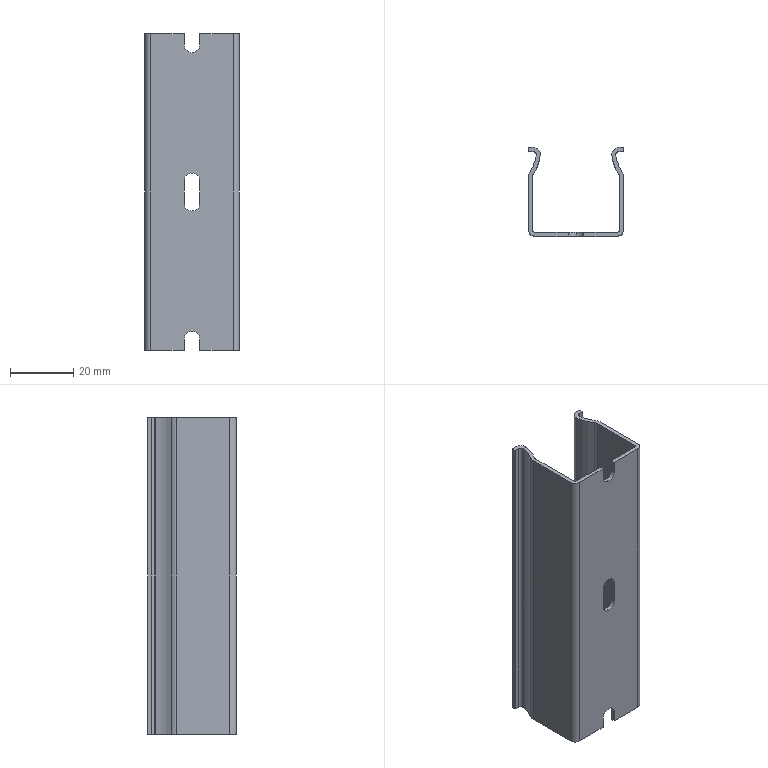Part | SolidWorks | features BaseBody 1 | 1 solid | 46 faces | box 30 x 28 x 100 mm | volume 10719 mm3 | cylinder 24 | plane 22 | commonest cylinder face diameters 5 x6 2 x3 4.5 x3 1.5 x2 3.5 x2 4 x2
STEP:
#1=CARTESIAN_POINT('',(-2.5,-14.,-100.));
#2=VERTEX_POINT('',#1);
#3=CARTESIAN_POINT('',(-2.5,-12.75,-100.));
#4=VERTEX_POINT('',#3);
#5=CARTESIAN_POINT('',(-2.5,14.001,-100.));
#6=DIRECTION('',(0.,1.,0.));
#7=VECTOR('',#6,1000.);
#8=LINE('',#5,#7);
#9=EDGE_CURVE('',#2,#4,#8,.T.);
#10=ORIENTED_EDGE('',*,*,#9,.T.);
#11=CARTESIAN_POINT('',(-2.5,-12.75,-96.5));
#12=VERTEX_POINT('',#11);
#13=CARTESIAN_POINT('',(-2.5,-12.75,-96.5));
#14=DIRECTION('',(0.,0.,1.));
#15=VECTOR('',#14,1000.);
#16=LINE('',#13,#15);
#17=EDGE_CURVE('',#4,#12,#16,.T.);
#18=ORIENTED_EDGE('',*,*,#17,.T.);
#19=CARTESIAN_POINT('',(-2.5,-14.,-96.5));
#20=VERTEX_POINT('',#19);
#21=CARTESIAN_POINT('',(-2.5,14.001,-96.5));
#22=DIRECTION('',(0.,-1.,0.));
#23=VECTOR('',#22,1000.);
#24=LINE('',#21,#23);
#25=EDGE_CURVE('',#12,#20,#24,.T.);
#26=ORIENTED_EDGE('',*,*,#25,.T.);
#27=CARTESIAN_POINT('',(-2.5,-14.,-96.5));
#28=DIRECTION('',(0.,0.,-1.));
#29=VECTOR('',#28,1000.);
#30=LINE('',#27,#29);
#31=EDGE_CURVE('',#20,#2,#30,.T.);
#32=ORIENTED_EDGE('',*,*,#31,.T.);
#33=EDGE_LOOP('',(#10,#18,#26,#32));
#34=FACE_OUTER_BOUND('',#33,.T.);
#35=CARTESIAN_POINT('',(-2.5,14.001,-96.5));
#36=DIRECTION('',(-1.,0.,0.));
#37=DIRECTION('',(0.,0.,1.));
#38=AXIS2_PLACEMENT_3D('',#35,#36,#37);
#39=PLANE('',#38);
#40=ADVANCED_FACE('',(#34),#39,.F.);
#41=CARTESIAN_POINT('',(2.5,-12.75,-100.));
#42=VERTEX_POINT('',#41);
#43=CARTESIAN_POINT('',(2.5,-14.,-100.));
#44=VERTEX_POINT('',#43);
#45=CARTESIAN_POINT('',(2.5,14.001,-100.));
#46=DIRECTION('',(0.,-1.,0.));
#47=VECTOR('',#46,1000.);
#48=LINE('',#45,#47);
#49=EDGE_CURVE('',#42,#44,#48,.T.);
#50=ORIENTED_EDGE('',*,*,#49,.T.);
#51=CARTESIAN_POINT('',(2.5,-14.,-96.5));
#52=VERTEX_POINT('',#51);
#53=CARTESIAN_POINT('',(2.5,-14.,-96.5));
#54=DIRECTION('',(0.,0.,1.));
#55=VECTOR('',#54,1000.);
#56=LINE('',#53,#55);
#57=EDGE_CURVE('',#44,#52,#56,.T.);
#58=ORIENTED_EDGE('',*,*,#57,.T.);
#59=CARTESIAN_POINT('',(2.5,-12.75,-96.5));
#60=VERTEX_POINT('',#59);
#61=CARTESIAN_POINT('',(2.5,14.001,-96.5));
#62=DIRECTION('',(0.,-1.,0.));
#63=VECTOR('',#62,1000.);
#64=LINE('',#61,#63);
#65=EDGE_CURVE('',#60,#52,#64,.T.);
#66=ORIENTED_EDGE('',*,*,#65,.F.);
#67=CARTESIAN_POINT('',(2.5,-12.75,-96.5));
#68=DIRECTION('',(0.,0.,-1.));
#69=VECTOR('',#68,1000.);
#70=LINE('',#67,#69);
#71=EDGE_CURVE('',#60,#42,#70,.T.);
#72=ORIENTED_EDGE('',*,*,#71,.T.);
#73=EDGE_LOOP('',(#50,#58,#66,#72));
#74=FACE_OUTER_BOUND('',#73,.T.);
#75=CARTESIAN_POINT('',(2.5,14.001,-96.5));
#76=DIRECTION('',(1.,0.,0.));
#77=DIRECTION('',(0.,0.,1.));
#78=AXIS2_PLACEMENT_3D('',#75,#76,#77);
#79=PLANE('',#78);
#80=ADVANCED_FACE('',(#74),#79,.F.);
#81=CARTESIAN_POINT('',(0.,-12.75,-96.5));
#82=DIRECTION('',(0.,1.,0.));
#83=DIRECTION('',(0.,0.,-1.));
#84=AXIS2_PLACEMENT_3D('',#81,#82,#83);
#85=CIRCLE('',#84,2.5);
#86=EDGE_CURVE('',#12,#60,#85,.T.);
#87=ORIENTED_EDGE('',*,*,#86,.T.);
#88=ORIENTED_EDGE('',*,*,#65,.T.);
#89=CARTESIAN_POINT('',(0.,-14.,-96.5));
#90=DIRECTION('',(0.,-1.,0.));
#91=DIRECTION('',(0.,0.,-1.));
#92=AXIS2_PLACEMENT_3D('',#89,#90,#91);
#93=CIRCLE('',#92,2.5);
#94=EDGE_CURVE('',#52,#20,#93,.T.);
#95=ORIENTED_EDGE('',*,*,#94,.T.);
#96=ORIENTED_EDGE('',*,*,#25,.F.);
#97=EDGE_LOOP('',(#87,#88,#95,#96));
#98=FACE_OUTER_BOUND('',#97,.T.);
#99=CARTESIAN_POINT('',(0.,14.001,-96.5));
#100=DIRECTION('',(0.,-1.,0.));
#101=DIRECTION('',(0.,0.,-1.));
#102=AXIS2_PLACEMENT_3D('',#99,#100,#101);
#103=CYLINDRICAL_SURFACE('',#102,2.5);
#104=ADVANCED_FACE('',(#98),#103,.F.);
#105=CARTESIAN_POINT('',(-2.5,-12.75,-53.5));
#106=VERTEX_POINT('',#105);
#107=CARTESIAN_POINT('',(-2.5,-12.75,-46.5));
#108=VERTEX_POINT('',#107);
#109=CARTESIAN_POINT('',(-2.5,-12.75,-46.5));
#110=DIRECTION('',(0.,0.,1.));
#111=VECTOR('',#110,1000.);
#112=LINE('',#109,#111);
#113=EDGE_CURVE('',#106,#108,#112,.T.);
#114=ORIENTED_EDGE('',*,*,#113,.T.);
#115=CARTESIAN_POINT('',(-2.5,-14.,-46.5));
#116=VERTEX_POINT('',#115);
#117=CARTESIAN_POINT('',(-2.5,14.001,-46.5));
#118=DIRECTION('',(0.,-1.,0.));
#119=VECTOR('',#118,1000.);
#120=LINE('',#117,#119);
#121=EDGE_CURVE('',#108,#116,#120,.T.);
#122=ORIENTED_EDGE('',*,*,#121,.T.);
#123=CARTESIAN_POINT('',(-2.5,-14.,-53.5));
#124=VERTEX_POINT('',#123);
#125=CARTESIAN_POINT('',(-2.5,-14.,-46.5));
#126=DIRECTION('',(0.,0.,-1.));
#127=VECTOR('',#126,1000.);
#128=LINE('',#125,#127);
#129=EDGE_CURVE('',#116,#124,#128,.T.);
#130=ORIENTED_EDGE('',*,*,#129,.T.);
#131=CARTESIAN_POINT('',(-2.5,14.001,-53.5));
#132=DIRECTION('',(0.,-1.,0.));
#133=VECTOR('',#132,1000.);
#134=LINE('',#131,#133);
#135=EDGE_CURVE('',#106,#124,#134,.T.);
#136=ORIENTED_EDGE('',*,*,#135,.F.);
#137=EDGE_LOOP('',(#114,#122,#130,#136));
#138=FACE_OUTER_BOUND('',#137,.T.);
#139=CARTESIAN_POINT('',(-2.5,14.001,-46.5));
#140=DIRECTION('',(-1.,0.,0.));
#141=DIRECTION('',(0.,0.,1.));
#142=AXIS2_PLACEMENT_3D('',#139,#140,#141);
#143=PLANE('',#142);
#144=ADVANCED_FACE('',(#138),#143,.F.);
#145=CARTESIAN_POINT('',(0.,-12.75,-56.));
#146=VERTEX_POINT('',#145);
#147=CARTESIAN_POINT('',(0.,-14.,-56.));
#148=VERTEX_POINT('',#147);
#149=CARTESIAN_POINT('',(0.,14.001,-56.));
#150=DIRECTION('',(0.,-1.,0.));
#151=VECTOR('',#150,1000.);
#152=LINE('',#149,#151);
#153=EDGE_CURVE('',#146,#148,#152,.T.);
#154=ORIENTED_EDGE('',*,*,#153,.F.);
#155=CARTESIAN_POINT('',(0.,-12.75,-53.5));
#156=DIRECTION('',(0.,1.,0.));
#157=DIRECTION('',(0.,0.,-1.));
#158=AXIS2_PLACEMENT_3D('',#155,#156,#157);
#159=CIRCLE('',#158,2.5);
#160=EDGE_CURVE('',#146,#106,#159,.T.);
#161=ORIENTED_EDGE('',*,*,#160,.T.);
#162=ORIENTED_EDGE('',*,*,#135,.T.);
#163=CARTESIAN_POINT('',(0.,-14.,-53.5));
#164=DIRECTION('',(0.,-1.,0.));
#165=DIRECTION('',(0.,0.,-1.));
#166=AXIS2_PLACEMENT_3D('',#163,#164,#165);
#167=CIRCLE('',#166,2.5);
#168=EDGE_CURVE('',#124,#148,#167,.T.);
#169=ORIENTED_EDGE('',*,*,#168,.T.);
#170=EDGE_LOOP('',(#154,#161,#162,#169));
#171=FACE_OUTER_BOUND('',#170,.T.);
#172=CARTESIAN_POINT('',(0.,14.001,-53.5));
#173=DIRECTION('',(0.,-1.,0.));
#174=DIRECTION('',(0.,0.,-1.));
#175=AXIS2_PLACEMENT_3D('',#172,#173,#174);
#176=CYLINDRICAL_SURFACE('',#175,2.5);
#177=ADVANCED_FACE('',(#171),#176,.F.);
#178=CARTESIAN_POINT('',(2.5,-12.75,-46.5));
#179=VERTEX_POINT('',#178);
#180=CARTESIAN_POINT('',(2.5,-12.75,-53.5));
#181=VERTEX_POINT('',#180);
#182=CARTESIAN_POINT('',(2.5,-12.75,-46.5));
#183=DIRECTION('',(0.,0.,-1.));
#184=VECTOR('',#183,1000.);
#185=LINE('',#182,#184);
#186=EDGE_CURVE('',#179,#181,#185,.T.);
#187=ORIENTED_EDGE('',*,*,#186,.T.);
#188=CARTESIAN_POINT('',(2.5,-14.,-53.5));
#189=VERTEX_POINT('',#188);
#190=CARTESIAN_POINT('',(2.5,14.001,-53.5));
#191=DIRECTION('',(0.,-1.,0.));
#192=VECTOR('',#191,1000.);
#193=LINE('',#190,#192);
#194=EDGE_CURVE('',#181,#189,#193,.T.);
#195=ORIENTED_EDGE('',*,*,#194,.T.);
#196=CARTESIAN_POINT('',(2.5,-14.,-46.5));
#197=VERTEX_POINT('',#196);
#198=CARTESIAN_POINT('',(2.5,-14.,-46.5));
#199=DIRECTION('',(0.,0.,1.));
#200=VECTOR('',#199,1000.);
#201=LINE('',#198,#200);
#202=EDGE_CURVE('',#189,#197,#201,.T.);
#203=ORIENTED_EDGE('',*,*,#202,.T.);
#204=CARTESIAN_POINT('',(2.5,14.001,-46.5));
#205=DIRECTION('',(0.,-1.,0.));
#206=VECTOR('',#205,1000.);
#207=LINE('',#204,#206);
#208=EDGE_CURVE('',#179,#197,#207,.T.);
#209=ORIENTED_EDGE('',*,*,#208,.F.);
#210=EDGE_LOOP('',(#187,#195,#203,#209));
#211=FACE_OUTER_BOUND('',#210,.T.);
#212=CARTESIAN_POINT('',(2.5,14.001,-46.5));
#213=DIRECTION('',(1.,0.,0.));
#214=DIRECTION('',(0.,0.,1.));
#215=AXIS2_PLACEMENT_3D('',#212,#213,#214);
#216=PLANE('',#215);
#217=ADVANCED_FACE('',(#211),#216,.F.);
#218=CARTESIAN_POINT('',(0.,-12.75,-46.5));
#219=DIRECTION('',(0.,1.,0.));
#220=DIRECTION('',(0.,0.,-1.));
#221=AXIS2_PLACEMENT_3D('',#218,#219,#220);
#222=CIRCLE('',#221,2.5);
#223=EDGE_CURVE('',#108,#179,#222,.T.);
#224=ORIENTED_EDGE('',*,*,#223,.T.);
#225=ORIENTED_EDGE('',*,*,#208,.T.);
#226=CARTESIAN_POINT('',(0.,-14.,-46.5));
#227=DIRECTION('',(0.,-1.,0.));
#228=DIRECTION('',(0.,0.,-1.));
#229=AXIS2_PLACEMENT_3D('',#226,#227,#228);
#230=CIRCLE('',#229,2.5);
#231=EDGE_CURVE('',#197,#116,#230,.T.);
#232=ORIENTED_EDGE('',*,*,#231,.T.);
#233=ORIENTED_EDGE('',*,*,#121,.F.);
#234=EDGE_LOOP('',(#224,#225,#232,#233));
#235=FACE_OUTER_BOUND('',#234,.T.);
#236=CARTESIAN_POINT('',(0.,14.001,-46.5));
#237=DIRECTION('',(0.,-1.,0.));
#238=DIRECTION('',(0.,0.,-1.));
#239=AXIS2_PLACEMENT_3D('',#236,#237,#238);
#240=CYLINDRICAL_SURFACE('',#239,2.5);
#241=ADVANCED_FACE('',(#235),#240,.F.);
#242=CARTESIAN_POINT('',(-2.5,-14.,0.));
#243=VERTEX_POINT('',#242);
#244=CARTESIAN_POINT('',(-2.5,-14.,-3.5));
#245=VERTEX_POINT('',#244);
#246=CARTESIAN_POINT('',(-2.5,-14.,3.5));
#247=DIRECTION('',(0.,0.,-1.));
#248=VECTOR('',#247,1000.);
#249=LINE('',#246,#248);
#250=EDGE_CURVE('',#243,#245,#249,.T.);
#251=ORIENTED_EDGE('',*,*,#250,.T.);
#252=CARTESIAN_POINT('',(-2.5,-12.75,-3.5));
#253=VERTEX_POINT('',#252);
#254=CARTESIAN_POINT('',(-2.5,14.001,-3.5));
#255=DIRECTION('',(0.,-1.,0.));
#256=VECTOR('',#255,1000.);
#257=LINE('',#254,#256);
#258=EDGE_CURVE('',#253,#245,#257,.T.);
#259=ORIENTED_EDGE('',*,*,#258,.F.);
#260=CARTESIAN_POINT('',(-2.5,-12.75,0.));
#261=VERTEX_POINT('',#260);
#262=CARTESIAN_POINT('',(-2.5,-12.75,3.5));
#263=DIRECTION('',(0.,0.,1.));
#264=VECTOR('',#263,1000.);
#265=LINE('',#262,#264);
#266=EDGE_CURVE('',#253,#261,#265,.T.);
#267=ORIENTED_EDGE('',*,*,#266,.T.);
#268=CARTESIAN_POINT('',(-2.5,14.001,0.));
#269=DIRECTION('',(0.,1.,0.));
#270=VECTOR('',#269,1000.);
#271=LINE('',#268,#270);
#272=EDGE_CURVE('',#243,#261,#271,.T.);
#273=ORIENTED_EDGE('',*,*,#272,.F.);
#274=EDGE_LOOP('',(#251,#259,#267,#273));
#275=FACE_OUTER_BOUND('',#274,.T.);
#276=CARTESIAN_POINT('',(-2.5,14.001,3.5));
#277=DIRECTION('',(-1.,0.,0.));
#278=DIRECTION('',(0.,0.,1.));
#279=AXIS2_PLACEMENT_3D('',#276,#277,#278);
#280=PLANE('',#279);
#281=ADVANCED_FACE('',(#275),#280,.F.);
#282=CARTESIAN_POINT('',(2.5,-12.75,0.));
#283=VERTEX_POINT('',#282);
#284=CARTESIAN_POINT('',(2.5,-12.75,-3.5));
#285=VERTEX_POINT('',#284);
#286=CARTESIAN_POINT('',(2.5,-12.75,3.5));
#287=DIRECTION('',(0.,0.,-1.));
#288=VECTOR('',#287,1000.);
#289=LINE('',#286,#288);
#290=EDGE_CURVE('',#283,#285,#289,.T.);
#291=ORIENTED_EDGE('',*,*,#290,.T.);
#292=CARTESIAN_POINT('',(2.5,-14.,-3.5));
#293=VERTEX_POINT('',#292);
#294=CARTESIAN_POINT('',(2.5,14.001,-3.5));
#295=DIRECTION('',(0.,-1.,0.));
#296=VECTOR('',#295,1000.);
#297=LINE('',#294,#296);
#298=EDGE_CURVE('',#285,#293,#297,.T.);
#299=ORIENTED_EDGE('',*,*,#298,.T.);
#300=CARTESIAN_POINT('',(2.5,-14.,0.));
#301=VERTEX_POINT('',#300);
#302=CARTESIAN_POINT('',(2.5,-14.,3.5));
#303=DIRECTION('',(0.,0.,1.));
#304=VECTOR('',#303,1000.);
#305=LINE('',#302,#304);
#306=EDGE_CURVE('',#293,#301,#305,.T.);
#307=ORIENTED_EDGE('',*,*,#306,.T.);
#308=CARTESIAN_POINT('',(2.5,14.001,0.));
#309=DIRECTION('',(0.,-1.,0.));
#310=VECTOR('',#309,1000.);
#311=LINE('',#308,#310);
#312=EDGE_CURVE('',#283,#301,#311,.T.);
#313=ORIENTED_EDGE('',*,*,#312,.F.);
#314=EDGE_LOOP('',(#291,#299,#307,#313));
#315=FACE_OUTER_BOUND('',#314,.T.);
#316=CARTESIAN_POINT('',(2.5,14.001,3.5));
#317=DIRECTION('',(1.,0.,0.));
#318=DIRECTION('',(0.,0.,1.));
#319=AXIS2_PLACEMENT_3D('',#316,#317,#318);
#320=PLANE('',#319);
#321=ADVANCED_FACE('',(#315),#320,.F.);
#322=CARTESIAN_POINT('',(0.,-12.75,-6.));
#323=VERTEX_POINT('',#322);
#324=CARTESIAN_POINT('',(0.,-14.,-6.));
#325=VERTEX_POINT('',#324);
#326=CARTESIAN_POINT('',(0.,14.001,-6.));
#327=DIRECTION('',(0.,-1.,0.));
#328=VECTOR('',#327,1000.);
#329=LINE('',#326,#328);
#330=EDGE_CURVE('',#323,#325,#329,.T.);
#331=ORIENTED_EDGE('',*,*,#330,.F.);
#332=CARTESIAN_POINT('',(0.,-12.75,-3.5));
#333=DIRECTION('',(0.,1.,0.));
#334=DIRECTION('',(0.,0.,-1.));
#335=AXIS2_PLACEMENT_3D('',#332,#333,#334);
#336=CIRCLE('',#335,2.5);
#337=EDGE_CURVE('',#323,#253,#336,.T.);
#338=ORIENTED_EDGE('',*,*,#337,.T.);
#339=ORIENTED_EDGE('',*,*,#258,.T.);
#340=CARTESIAN_POINT('',(0.,-14.,-3.5));
#341=DIRECTION('',(0.,-1.,0.));
#342=DIRECTION('',(0.,0.,-1.));
#343=AXIS2_PLACEMENT_3D('',#340,#341,#342);
#344=CIRCLE('',#343,2.5);
#345=EDGE_CURVE('',#245,#325,#344,.T.);
#346=ORIENTED_EDGE('',*,*,#345,.T.);
#347=EDGE_LOOP('',(#331,#338,#339,#346));
#348=FACE_OUTER_BOUND('',#347,.T.);
#349=CARTESIAN_POINT('',(0.,14.001,-3.5));
#350=DIRECTION('',(0.,-1.,0.));
#351=DIRECTION('',(0.,0.,-1.));
#352=AXIS2_PLACEMENT_3D('',#349,#350,#351);
#353=CYLINDRICAL_SURFACE('',#352,2.5);
#354=ADVANCED_FACE('',(#348),#353,.F.);
#355=CARTESIAN_POINT('',(-13.,-12.75,-100.));
#356=VERTEX_POINT('',#355);
#357=CARTESIAN_POINT('',(-13.75,-12.,-100.));
#358=VERTEX_POINT('',#357);
#359=CARTESIAN_POINT('',(-13.,-12.,-100.));
#360=DIRECTION('',(0.,0.,-1.));
#361=DIRECTION('',(1.,0.,0.));
#362=AXIS2_PLACEMENT_3D('',#359,#360,#361);
#363=CIRCLE('',#362,0.75);
#364=EDGE_CURVE('',#356,#358,#363,.T.);
#365=ORIENTED_EDGE('',*,*,#364,.T.);
#366=CARTESIAN_POINT('',(-13.75,-12.,0.));
#367=VERTEX_POINT('',#366);
#368=CARTESIAN_POINT('',(-13.75,-12.,-100.));
#369=DIRECTION('',(0.,0.,1.));
#370=VECTOR('',#369,1000.);
#371=LINE('',#368,#370);
#372=EDGE_CURVE('',#358,#367,#371,.T.);
#373=ORIENTED_EDGE('',*,*,#372,.T.);
#374=CARTESIAN_POINT('',(-13.,-12.75,0.));
#375=VERTEX_POINT('',#374);
#376=CARTESIAN_POINT('',(-13.,-12.,0.));
#377=DIRECTION('',(0.,0.,1.));
#378=DIRECTION('',(1.,0.,0.));
#379=AXIS2_PLACEMENT_3D('',#376,#377,#378);
#380=CIRCLE('',#379,0.75);
#381=EDGE_CURVE('',#367,#375,#380,.T.);
#382=ORIENTED_EDGE('',*,*,#381,.T.);
#383=CARTESIAN_POINT('',(-13.,-12.75,-100.));
#384=DIRECTION('',(0.,0.,-1.));
#385=VECTOR('',#384,1000.);
#386=LINE('',#383,#385);
#387=EDGE_CURVE('',#375,#356,#386,.T.);
#388=ORIENTED_EDGE('',*,*,#387,.T.);
#389=EDGE_LOOP('',(#365,#373,#382,#388));
#390=FACE_OUTER_BOUND('',#389,.T.);
#391=CARTESIAN_POINT('',(-13.,-12.,-100.));
#392=DIRECTION('',(0.,0.,1.));
#393=DIRECTION('',(1.,0.,0.));
#394=AXIS2_PLACEMENT_3D('',#391,#392,#393);
#395=CYLINDRICAL_SURFACE('',#394,0.75);
#396=ADVANCED_FACE('',(#390),#395,.F.);
#397=CARTESIAN_POINT('',(13.75,-12.,-100.));
#398=VERTEX_POINT('',#397);
#399=CARTESIAN_POINT('',(13.,-12.75,-100.));
#400=VERTEX_POINT('',#399);
#401=CARTESIAN_POINT('',(13.,-12.,-100.));
#402=DIRECTION('',(0.,0.,-1.));
#403=DIRECTION('',(1.,0.,0.));
#404=AXIS2_PLACEMENT_3D('',#401,#402,#403);
#405=CIRCLE('',#404,0.75);
#406=EDGE_CURVE('',#398,#400,#405,.T.);
#407=ORIENTED_EDGE('',*,*,#406,.T.);
#408=CARTESIAN_POINT('',(13.,-12.75,0.));
#409=VERTEX_POINT('',#408);
#410=CARTESIAN_POINT('',(13.,-12.75,-100.));
#411=DIRECTION('',(0.,0.,1.));
#412=VECTOR('',#411,1000.);
#413=LINE('',#410,#412);
#414=EDGE_CURVE('',#400,#409,#413,.T.);
#415=ORIENTED_EDGE('',*,*,#414,.T.);
#416=CARTESIAN_POINT('',(13.75,-12.,0.));
#417=VERTEX_POINT('',#416);
#418=CARTESIAN_POINT('',(13.,-12.,0.));
#419=DIRECTION('',(0.,0.,1.));
#420=DIRECTION('',(1.,0.,0.));
#421=AXIS2_PLACEMENT_3D('',#418,#419,#420);
#422=CIRCLE('',#421,0.75);
#423=EDGE_CURVE('',#409,#417,#422,.T.);
#424=ORIENTED_EDGE('',*,*,#423,.T.);
#425=CARTESIAN_POINT('',(13.75,-12.,-100.));
#426=DIRECTION('',(0.,0.,-1.));
#427=VECTOR('',#426,1000.);
#428=LINE('',#425,#427);
#429=EDGE_CURVE('',#417,#398,#428,.T.);
#430=ORIENTED_EDGE('',*,*,#429,.T.);
#431=EDGE_LOOP('',(#407,#415,#424,#430));
#432=FACE_OUTER_BOUND('',#431,.T.);
#433=CARTESIAN_POINT('',(13.,-12.,-100.));
#434=DIRECTION('',(0.,0.,1.));
#435=DIRECTION('',(1.,0.,0.));
#436=AXIS2_PLACEMENT_3D('',#433,#434,#435);
#437=CYLINDRICAL_SURFACE('',#436,0.75);
#438=ADVANCED_FACE('',(#432),#437,.F.);
#439=CARTESIAN_POINT('',(13.439,5.746,-100.));
#440=VERTEX_POINT('',#439);
#441=CARTESIAN_POINT('',(13.75,4.75,-100.));
#442=VERTEX_POINT('',#441);
#443=CARTESIAN_POINT('',(12.,4.75,-100.));
#444=DIRECTION('',(0.,0.,-1.));
#445=DIRECTION('',(1.,0.,0.));
#446=AXIS2_PLACEMENT_3D('',#443,#444,#445);
#447=CIRCLE('',#446,1.75);
#448=EDGE_CURVE('',#440,#442,#447,.T.);
#449=ORIENTED_EDGE('',*,*,#448,.T.);
#450=CARTESIAN_POINT('',(13.75,4.75,0.));
#451=VERTEX_POINT('',#450);
#452=CARTESIAN_POINT('',(13.75,4.75,-100.));
#453=DIRECTION('',(0.,0.,1.));
#454=VECTOR('',#453,1000.);
#455=LINE('',#452,#454);
#456=EDGE_CURVE('',#442,#451,#455,.T.);
#457=ORIENTED_EDGE('',*,*,#456,.T.);
#458=CARTESIAN_POINT('',(13.439,5.746,0.));
#459=VERTEX_POINT('',#458);
#460=CARTESIAN_POINT('',(12.,4.75,0.));
#461=DIRECTION('',(0.,0.,1.));
#462=DIRECTION('',(1.,0.,0.));
#463=AXIS2_PLACEMENT_3D('',#460,#461,#462);
#464=CIRCLE('',#463,1.75);
#465=EDGE_CURVE('',#451,#459,#464,.T.);
#466=ORIENTED_EDGE('',*,*,#465,.T.);
#467=CARTESIAN_POINT('',(13.439,5.746,-100.));
#468=DIRECTION('',(0.,0.,-1.));
#469=VECTOR('',#468,1000.);
#470=LINE('',#467,#469);
#471=EDGE_CURVE('',#459,#440,#470,.T.);
#472=ORIENTED_EDGE('',*,*,#471,.T.);
#473=EDGE_LOOP('',(#449,#457,#466,#472));
#474=FACE_OUTER_BOUND('',#473,.T.);
#475=CARTESIAN_POINT('',(12.,4.75,-100.));
#476=DIRECTION('',(0.,0.,1.));
#477=DIRECTION('',(1.,0.,0.));
#478=AXIS2_PLACEMENT_3D('',#475,#476,#477);
#479=CYLINDRICAL_SURFACE('',#478,1.75);
#480=ADVANCED_FACE('',(#474),#479,.F.);
#481=CARTESIAN_POINT('',(-13.75,4.75,-100.));
#482=VERTEX_POINT('',#481);
#483=CARTESIAN_POINT('',(-13.439,5.746,-100.));
#484=VERTEX_POINT('',#483);
#485=CARTESIAN_POINT('',(-12.,4.75,-100.));
#486=DIRECTION('',(0.,0.,-1.));
#487=DIRECTION('',(1.,0.,0.));
#488=AXIS2_PLACEMENT_3D('',#485,#486,#487);
#489=CIRCLE('',#488,1.75);
#490=EDGE_CURVE('',#482,#484,#489,.T.);
#491=ORIENTED_EDGE('',*,*,#490,.T.);
#492=CARTESIAN_POINT('',(-13.439,5.746,0.));
#493=VERTEX_POINT('',#492);
#494=CARTESIAN_POINT('',(-13.439,5.746,-100.));
#495=DIRECTION('',(0.,0.,1.));
#496=VECTOR('',#495,1000.);
#497=LINE('',#494,#496);
#498=EDGE_CURVE('',#484,#493,#497,.T.);
#499=ORIENTED_EDGE('',*,*,#498,.T.);
#500=CARTESIAN_POINT('',(-13.75,4.75,0.));
#501=VERTEX_POINT('',#500);
#502=CARTESIAN_POINT('',(-12.,4.75,0.));
#503=DIRECTION('',(0.,0.,1.));
#504=DIRECTION('',(1.,0.,0.));
#505=AXIS2_PLACEMENT_3D('',#502,#503,#504);
#506=CIRCLE('',#505,1.75);
#507=EDGE_CURVE('',#493,#501,#506,.T.);
#508=ORIENTED_EDGE('',*,*,#507,.T.);
#509=CARTESIAN_POINT('',(-13.75,4.75,-100.));
#510=DIRECTION('',(0.,0.,-1.));
#511=VECTOR('',#510,1000.);
#512=LINE('',#509,#511);
#513=EDGE_CURVE('',#501,#482,#512,.T.);
#514=ORIENTED_EDGE('',*,*,#513,.T.);
#515=EDGE_LOOP('',(#491,#499,#508,#514));
#516=FACE_OUTER_BOUND('',#515,.T.);
#517=CARTESIAN_POINT('',(-12.,4.75,-100.));
#518=DIRECTION('',(0.,0.,1.));
#519=DIRECTION('',(1.,0.,0.));
#520=AXIS2_PLACEMENT_3D('',#517,#518,#519);
#521=CYLINDRICAL_SURFACE('',#520,1.75);
#522=ADVANCED_FACE('',(#516),#521,.F.);
#523=CARTESIAN_POINT('',(13.55,14.,-100.));
#524=VERTEX_POINT('',#523);
#525=CARTESIAN_POINT('',(11.311,11.526,-100.));
#526=VERTEX_POINT('',#525);
#527=CARTESIAN_POINT('',(13.55,11.75,-100.));
#528=DIRECTION('',(0.,0.,1.));
#529=DIRECTION('',(1.,0.,0.));
#530=AXIS2_PLACEMENT_3D('',#527,#528,#529);
#531=CIRCLE('',#530,2.25);
#532=EDGE_CURVE('',#524,#526,#531,.T.);
#533=ORIENTED_EDGE('',*,*,#532,.T.);
#534=CARTESIAN_POINT('',(11.311,11.526,0.));
#535=VERTEX_POINT('',#534);
#536=CARTESIAN_POINT('',(11.311,11.526,-100.));
#537=DIRECTION('',(0.,0.,1.));
#538=VECTOR('',#537,1000.);
#539=LINE('',#536,#538);
#540=EDGE_CURVE('',#526,#535,#539,.T.);
#541=ORIENTED_EDGE('',*,*,#540,.T.);
#542=CARTESIAN_POINT('',(13.55,14.,0.));
#543=VERTEX_POINT('',#542);
#544=CARTESIAN_POINT('',(13.55,11.75,0.));
#545=DIRECTION('',(0.,0.,-1.));
#546=DIRECTION('',(1.,0.,0.));
#547=AXIS2_PLACEMENT_3D('',#544,#545,#546);
#548=CIRCLE('',#547,2.25);
#549=EDGE_CURVE('',#535,#543,#548,.T.);
#550=ORIENTED_EDGE('',*,*,#549,.T.);
#551=CARTESIAN_POINT('',(13.55,14.,-100.));
#552=DIRECTION('',(0.,0.,-1.));
#553=VECTOR('',#552,1000.);
#554=LINE('',#551,#553);
#555=EDGE_CURVE('',#543,#524,#554,.T.);
#556=ORIENTED_EDGE('',*,*,#555,.T.);
#557=EDGE_LOOP('',(#533,#541,#550,#556));
#558=FACE_OUTER_BOUND('',#557,.T.);
#559=CARTESIAN_POINT('',(13.55,11.75,-100.));
#560=DIRECTION('',(0.,0.,1.));
#561=DIRECTION('',(1.,0.,0.));
#562=AXIS2_PLACEMENT_3D('',#559,#560,#561);
#563=CYLINDRICAL_SURFACE('',#562,2.25);
#564=ADVANCED_FACE('',(#558),#563,.T.);
#565=CARTESIAN_POINT('',(-11.3,11.75,-100.));
#566=VERTEX_POINT('',#565);
#567=CARTESIAN_POINT('',(-11.3,11.75,0.));
#568=VERTEX_POINT('',#567);
#569=CARTESIAN_POINT('',(-11.3,11.75,-100.));
#570=DIRECTION('',(0.,0.,1.));
#571=VECTOR('',#570,1000.);
#572=LINE('',#569,#571);
#573=EDGE_CURVE('',#566,#568,#572,.T.);
#574=ORIENTED_EDGE('',*,*,#573,.F.);
#575=CARTESIAN_POINT('',(-13.55,14.,-100.));
#576=VERTEX_POINT('',#575);
#577=CARTESIAN_POINT('',(-13.55,11.75,-100.));
#578=DIRECTION('',(0.,0.,1.));
#579=DIRECTION('',(1.,0.,0.));
#580=AXIS2_PLACEMENT_3D('',#577,#578,#579);
#581=CIRCLE('',#580,2.25);
#582=EDGE_CURVE('',#566,#576,#581,.T.);
#583=ORIENTED_EDGE('',*,*,#582,.T.);
#584=CARTESIAN_POINT('',(-13.55,14.,0.));
#585=VERTEX_POINT('',#584);
#586=CARTESIAN_POINT('',(-13.55,14.,-100.));
#587=DIRECTION('',(0.,0.,1.));
#588=VECTOR('',#587,1000.);
#589=LINE('',#586,#588);
#590=EDGE_CURVE('',#576,#585,#589,.T.);
#591=ORIENTED_EDGE('',*,*,#590,.T.);
#592=CARTESIAN_POINT('',(-13.55,11.75,0.));
#593=DIRECTION('',(0.,0.,-1.));
#594=DIRECTION('',(1.,0.,0.));
#595=AXIS2_PLACEMENT_3D('',#592,#593,#594);
#596=CIRCLE('',#595,2.25);
#597=EDGE_CURVE('',#585,#568,#596,.T.);
#598=ORIENTED_EDGE('',*,*,#597,.T.);
#599=EDGE_LOOP('',(#574,#583,#591,#598));
#600=FACE_OUTER_BOUND('',#599,.T.);
#601=CARTESIAN_POINT('',(-13.55,11.75,-100.));
#602=DIRECTION('',(0.,0.,1.));
#603=DIRECTION('',(1.,0.,0.));
#604=AXIS2_PLACEMENT_3D('',#601,#602,#603);
#605=CYLINDRICAL_SURFACE('',#604,2.25);
#606=ADVANCED_FACE('',(#600),#605,.T.);
#607=CARTESIAN_POINT('',(-11.311,11.526,-100.));
#608=VERTEX_POINT('',#607);
#609=CARTESIAN_POINT('',(-23.55,12.75,-100.));
#610=DIRECTION('',(0.,0.,1.));
#611=DIRECTION('',(1.,0.,0.));
#612=AXIS2_PLACEMENT_3D('',#609,#610,#611);
#613=CIRCLE('',#612,12.3);
#614=EDGE_CURVE('',#484,#608,#613,.T.);
#615=ORIENTED_EDGE('',*,*,#614,.T.);
#616=CARTESIAN_POINT('',(-11.311,11.526,0.));
#617=VERTEX_POINT('',#616);
#618=CARTESIAN_POINT('',(-11.311,11.526,-100.));
#619=DIRECTION('',(0.,0.,-1.));
#620=VECTOR('',#619,1000.);
#621=LINE('',#618,#620);
#622=EDGE_CURVE('',#617,#608,#621,.T.);
#623=ORIENTED_EDGE('',*,*,#622,.F.);
#624=CARTESIAN_POINT('',(-23.55,12.75,0.));
#625=DIRECTION('',(0.,0.,1.));
#626=DIRECTION('',(1.,0.,0.));
#627=AXIS2_PLACEMENT_3D('',#624,#625,#626);
#628=CIRCLE('',#627,12.3);
#629=EDGE_CURVE('',#493,#617,#628,.T.);
#630=ORIENTED_EDGE('',*,*,#629,.F.);
#631=ORIENTED_EDGE('',*,*,#498,.F.);
#632=EDGE_LOOP('',(#615,#623,#630,#631));
#633=FACE_OUTER_BOUND('',#632,.T.);
#634=CARTESIAN_POINT('',(-23.55,12.75,-100.));
#635=DIRECTION('',(0.,0.,1.));
#636=DIRECTION('',(1.,0.,0.));
#637=AXIS2_PLACEMENT_3D('',#634,#635,#636);
#638=CYLINDRICAL_SURFACE('',#637,12.3);
#639=ADVANCED_FACE('',(#633),#638,.T.);
#640=CARTESIAN_POINT('',(23.55,12.75,0.));
#641=DIRECTION('',(0.,0.,1.));
#642=DIRECTION('',(1.,0.,0.));
#643=AXIS2_PLACEMENT_3D('',#640,#641,#642);
#644=CIRCLE('',#643,12.3);
#645=EDGE_CURVE('',#535,#459,#644,.T.);
#646=ORIENTED_EDGE('',*,*,#645,.F.);
#647=ORIENTED_EDGE('',*,*,#540,.F.);
#648=CARTESIAN_POINT('',(23.55,12.75,-100.));
#649=DIRECTION('',(0.,0.,1.));
#650=DIRECTION('',(1.,0.,0.));
#651=AXIS2_PLACEMENT_3D('',#648,#649,#650);
#652=CIRCLE('',#651,12.3);
#653=EDGE_CURVE('',#526,#440,#652,.T.);
#654=ORIENTED_EDGE('',*,*,#653,.T.);
#655=ORIENTED_EDGE('',*,*,#471,.F.);
#656=EDGE_LOOP('',(#646,#647,#654,#655));
#657=FACE_OUTER_BOUND('',#656,.T.);
#658=CARTESIAN_POINT('',(23.55,12.75,-100.));
#659=DIRECTION('',(0.,0.,1.));
#660=DIRECTION('',(1.,0.,0.));
#661=AXIS2_PLACEMENT_3D('',#658,#659,#660);
#662=CYLINDRICAL_SURFACE('',#661,12.3);
#663=ADVANCED_FACE('',(#657),#662,.T.);
#664=ORIENTED_EDGE('',*,*,#186,.F.);
#665=ORIENTED_EDGE('',*,*,#223,.F.);
#666=ORIENTED_EDGE('',*,*,#113,.F.);
#667=ORIENTED_EDGE('',*,*,#160,.F.);
#668=CARTESIAN_POINT('',(0.,-12.75,-53.5));
#669=DIRECTION('',(0.,1.,0.));
#670=DIRECTION('',(0.,0.,-1.));
#671=AXIS2_PLACEMENT_3D('',#668,#669,#670);
#672=CIRCLE('',#671,2.5);
#673=EDGE_CURVE('',#181,#146,#672,.T.);
#674=ORIENTED_EDGE('',*,*,#673,.F.);
#675=EDGE_LOOP('',(#664,#665,#666,#667,#674));
#676=FACE_BOUND('',#675,.T.);
#677=CARTESIAN_POINT('',(0.,-12.75,-100.));
#678=DIRECTION('',(1.,0.,0.));
#679=VECTOR('',#678,1000.);
#680=LINE('',#677,#679);
#681=EDGE_CURVE('',#42,#400,#680,.T.);
#682=ORIENTED_EDGE('',*,*,#681,.F.);
#683=ORIENTED_EDGE('',*,*,#71,.F.);
#684=ORIENTED_EDGE('',*,*,#86,.F.);
#685=ORIENTED_EDGE('',*,*,#17,.F.);
#686=CARTESIAN_POINT('',(0.,-12.75,-100.));
#687=DIRECTION('',(1.,0.,0.));
#688=VECTOR('',#687,1000.);
#689=LINE('',#686,#688);
#690=EDGE_CURVE('',#356,#4,#689,.T.);
#691=ORIENTED_EDGE('',*,*,#690,.F.);
#692=ORIENTED_EDGE('',*,*,#387,.F.);
#693=CARTESIAN_POINT('',(0.,-12.75,0.));
#694=DIRECTION('',(1.,0.,0.));
#695=VECTOR('',#694,1000.);
#696=LINE('',#693,#695);
#697=EDGE_CURVE('',#375,#261,#696,.T.);
#698=ORIENTED_EDGE('',*,*,#697,.T.);
#699=ORIENTED_EDGE('',*,*,#266,.F.);
#700=ORIENTED_EDGE('',*,*,#337,.F.);
#701=CARTESIAN_POINT('',(0.,-12.75,-3.5));
#702=DIRECTION('',(0.,1.,0.));
#703=DIRECTION('',(0.,0.,-1.));
#704=AXIS2_PLACEMENT_3D('',#701,#702,#703);
#705=CIRCLE('',#704,2.5);
#706=EDGE_CURVE('',#285,#323,#705,.T.);
#707=ORIENTED_EDGE('',*,*,#706,.F.);
#708=ORIENTED_EDGE('',*,*,#290,.F.);
#709=CARTESIAN_POINT('',(0.,-12.75,0.));
#710=DIRECTION('',(1.,0.,0.));
#711=VECTOR('',#710,1000.);
#712=LINE('',#709,#711);
#713=EDGE_CURVE('',#283,#409,#712,.T.);
#714=ORIENTED_EDGE('',*,*,#713,.T.);
#715=ORIENTED_EDGE('',*,*,#414,.F.);
#716=EDGE_LOOP('',(#682,#683,#684,#685,#691,#692,#698,#699,#700,#707,#708,#714,#715));
#717=FACE_OUTER_BOUND('',#716,.T.);
#718=CARTESIAN_POINT('',(-15.,-12.75,-100.));
#719=DIRECTION('',(0.,-1.,0.));
#720=DIRECTION('',(0.,0.,-1.));
#721=AXIS2_PLACEMENT_3D('',#718,#719,#720);
#722=PLANE('',#721);
#723=ADVANCED_FACE('',(#676,#717),#722,.F.);
#724=CARTESIAN_POINT('',(13.75,0.,0.));
#725=DIRECTION('',(0.,1.,0.));
#726=VECTOR('',#725,1000.);
#727=LINE('',#724,#726);
#728=EDGE_CURVE('',#417,#451,#727,.T.);
#729=ORIENTED_EDGE('',*,*,#728,.T.);
#730=ORIENTED_EDGE('',*,*,#456,.F.);
#731=CARTESIAN_POINT('',(13.75,0.,-100.));
#732=DIRECTION('',(0.,1.,0.));
#733=VECTOR('',#732,1000.);
#734=LINE('',#731,#733);
#735=EDGE_CURVE('',#398,#442,#734,.T.);
#736=ORIENTED_EDGE('',*,*,#735,.F.);
#737=ORIENTED_EDGE('',*,*,#429,.F.);
#738=EDGE_LOOP('',(#729,#730,#736,#737));
#739=FACE_OUTER_BOUND('',#738,.T.);
#740=CARTESIAN_POINT('',(13.75,14.,-100.));
#741=DIRECTION('',(1.,0.,0.));
#742=DIRECTION('',(0.,1.,0.));
#743=AXIS2_PLACEMENT_3D('',#740,#741,#742);
#744=PLANE('',#743);
#745=ADVANCED_FACE('',(#739),#744,.F.);
#746=CARTESIAN_POINT('',(-13.75,0.,-100.));
#747=DIRECTION('',(0.,-1.,0.));
#748=VECTOR('',#747,1000.);
#749=LINE('',#746,#748);
#750=EDGE_CURVE('',#482,#358,#749,.T.);
#751=ORIENTED_EDGE('',*,*,#750,.F.);
#752=ORIENTED_EDGE('',*,*,#513,.F.);
#753=CARTESIAN_POINT('',(-13.75,0.,0.));
#754=DIRECTION('',(0.,-1.,0.));
#755=VECTOR('',#754,1000.);
#756=LINE('',#753,#755);
#757=EDGE_CURVE('',#501,#367,#756,.T.);
#758=ORIENTED_EDGE('',*,*,#757,.T.);
#759=ORIENTED_EDGE('',*,*,#372,.F.);
#760=EDGE_LOOP('',(#751,#752,#758,#759));
#761=FACE_OUTER_BOUND('',#760,.T.);
#762=CARTESIAN_POINT('',(-13.75,14.,-100.));
#763=DIRECTION('',(-1.,0.,0.));
#764=DIRECTION('',(0.,1.,0.));
#765=AXIS2_PLACEMENT_3D('',#762,#763,#764);
#766=PLANE('',#765);
#767=ADVANCED_FACE('',(#761),#766,.F.);
#768=CARTESIAN_POINT('',(-13.,-14.,-100.));
#769=VERTEX_POINT('',#768);
#770=CARTESIAN_POINT('',(-15.,-12.,-100.));
#771=VERTEX_POINT('',#770);
#772=CARTESIAN_POINT('',(-13.,-12.,-100.));
#773=DIRECTION('',(0.,0.,-1.));
#774=DIRECTION('',(1.,0.,0.));
#775=AXIS2_PLACEMENT_3D('',#772,#773,#774);
#776=CIRCLE('',#775,2.);
#777=EDGE_CURVE('',#769,#771,#776,.T.);
#778=ORIENTED_EDGE('',*,*,#777,.F.);
#779=CARTESIAN_POINT('',(-13.,-14.,0.));
#780=VERTEX_POINT('',#779);
#781=CARTESIAN_POINT('',(-13.,-14.,-100.));
#782=DIRECTION('',(0.,0.,-1.));
#783=VECTOR('',#782,1000.);
#784=LINE('',#781,#783);
#785=EDGE_CURVE('',#780,#769,#784,.T.);
#786=ORIENTED_EDGE('',*,*,#785,.F.);
#787=CARTESIAN_POINT('',(-15.,-12.,0.));
#788=VERTEX_POINT('',#787);
#789=CARTESIAN_POINT('',(-13.,-12.,0.));
#790=DIRECTION('',(0.,0.,1.));
#791=DIRECTION('',(1.,0.,0.));
#792=AXIS2_PLACEMENT_3D('',#789,#790,#791);
#793=CIRCLE('',#792,2.);
#794=EDGE_CURVE('',#788,#780,#793,.T.);
#795=ORIENTED_EDGE('',*,*,#794,.F.);
#796=CARTESIAN_POINT('',(-15.,-12.,-100.));
#797=DIRECTION('',(0.,0.,1.));
#798=VECTOR('',#797,1000.);
#799=LINE('',#796,#798);
#800=EDGE_CURVE('',#771,#788,#799,.T.);
#801=ORIENTED_EDGE('',*,*,#800,.F.);
#802=EDGE_LOOP('',(#778,#786,#795,#801));
#803=FACE_OUTER_BOUND('',#802,.T.);
#804=CARTESIAN_POINT('',(-13.,-12.,-100.));
#805=DIRECTION('',(0.,0.,1.));
#806=DIRECTION('',(1.,0.,0.));
#807=AXIS2_PLACEMENT_3D('',#804,#805,#806);
#808=CYLINDRICAL_SURFACE('',#807,2.);
#809=ADVANCED_FACE('',(#803),#808,.T.);
#810=CARTESIAN_POINT('',(15.,-12.,-100.));
#811=VERTEX_POINT('',#810);
#812=CARTESIAN_POINT('',(13.,-14.,-100.));
#813=VERTEX_POINT('',#812);
#814=CARTESIAN_POINT('',(13.,-12.,-100.));
#815=DIRECTION('',(0.,0.,-1.));
#816=DIRECTION('',(1.,0.,0.));
#817=AXIS2_PLACEMENT_3D('',#814,#815,#816);
#818=CIRCLE('',#817,2.);
#819=EDGE_CURVE('',#811,#813,#818,.T.);
#820=ORIENTED_EDGE('',*,*,#819,.F.);
#821=CARTESIAN_POINT('',(15.,-12.,0.));
#822=VERTEX_POINT('',#821);
#823=CARTESIAN_POINT('',(15.,-12.,-100.));
#824=DIRECTION('',(0.,0.,-1.));
#825=VECTOR('',#824,1000.);
#826=LINE('',#823,#825);
#827=EDGE_CURVE('',#822,#811,#826,.T.);
#828=ORIENTED_EDGE('',*,*,#827,.F.);
#829=CARTESIAN_POINT('',(13.,-14.,0.));
#830=VERTEX_POINT('',#829);
#831=CARTESIAN_POINT('',(13.,-12.,0.));
#832=DIRECTION('',(0.,0.,1.));
#833=DIRECTION('',(1.,0.,0.));
#834=AXIS2_PLACEMENT_3D('',#831,#832,#833);
#835=CIRCLE('',#834,2.);
#836=EDGE_CURVE('',#830,#822,#835,.T.);
#837=ORIENTED_EDGE('',*,*,#836,.F.);
#838=CARTESIAN_POINT('',(13.,-14.,-100.));
#839=DIRECTION('',(0.,0.,1.));
#840=VECTOR('',#839,1000.);
#841=LINE('',#838,#840);
#842=EDGE_CURVE('',#813,#830,#841,.T.);
#843=ORIENTED_EDGE('',*,*,#842,.F.);
#844=EDGE_LOOP('',(#820,#828,#837,#843));
#845=FACE_OUTER_BOUND('',#844,.T.);
#846=CARTESIAN_POINT('',(13.,-12.,-100.));
#847=DIRECTION('',(0.,0.,1.));
#848=DIRECTION('',(1.,0.,0.));
#849=AXIS2_PLACEMENT_3D('',#846,#847,#848);
#850=CYLINDRICAL_SURFACE('',#849,2.);
#851=ADVANCED_FACE('',(#845),#850,.T.);
#852=CARTESIAN_POINT('',(14.466,6.458,-100.));
#853=VERTEX_POINT('',#852);
#854=CARTESIAN_POINT('',(15.,4.75,-100.));
#855=VERTEX_POINT('',#854);
#856=CARTESIAN_POINT('',(12.,4.75,-100.));
#857=DIRECTION('',(0.,0.,-1.));
#858=DIRECTION('',(1.,0.,0.));
#859=AXIS2_PLACEMENT_3D('',#856,#857,#858);
#860=CIRCLE('',#859,3.);
#861=EDGE_CURVE('',#853,#855,#860,.T.);
#862=ORIENTED_EDGE('',*,*,#861,.F.);
#863=CARTESIAN_POINT('',(14.466,6.458,0.));
#864=VERTEX_POINT('',#863);
#865=CARTESIAN_POINT('',(14.466,6.458,-100.));
#866=DIRECTION('',(0.,0.,-1.));
#867=VECTOR('',#866,1000.);
#868=LINE('',#865,#867);
#869=EDGE_CURVE('',#864,#853,#868,.T.);
#870=ORIENTED_EDGE('',*,*,#869,.F.);
#871=CARTESIAN_POINT('',(15.,4.75,0.));
#872=VERTEX_POINT('',#871);
#873=CARTESIAN_POINT('',(12.,4.75,0.));
#874=DIRECTION('',(0.,0.,1.));
#875=DIRECTION('',(1.,0.,0.));
#876=AXIS2_PLACEMENT_3D('',#873,#874,#875);
#877=CIRCLE('',#876,3.);
#878=EDGE_CURVE('',#872,#864,#877,.T.);
#879=ORIENTED_EDGE('',*,*,#878,.F.);
#880=CARTESIAN_POINT('',(15.,4.75,0.));
#881=DIRECTION('',(0.,0.,1.));
#882=VECTOR('',#881,1000.);
#883=LINE('',#880,#882);
#884=EDGE_CURVE('',#855,#872,#883,.T.);
#885=ORIENTED_EDGE('',*,*,#884,.F.);
#886=EDGE_LOOP('',(#862,#870,#879,#885));
#887=FACE_OUTER_BOUND('',#886,.T.);
#888=CARTESIAN_POINT('',(12.,4.75,-100.));
#889=DIRECTION('',(0.,0.,1.));
#890=DIRECTION('',(1.,0.,0.));
#891=AXIS2_PLACEMENT_3D('',#888,#889,#890);
#892=CYLINDRICAL_SURFACE('',#891,3.);
#893=ADVANCED_FACE('',(#887),#892,.T.);
#894=CARTESIAN_POINT('',(-15.,4.75,-100.));
#895=VERTEX_POINT('',#894);
#896=CARTESIAN_POINT('',(-14.466,6.458,-100.));
#897=VERTEX_POINT('',#896);
#898=CARTESIAN_POINT('',(-12.,4.75,-100.));
#899=DIRECTION('',(0.,0.,-1.));
#900=DIRECTION('',(1.,0.,0.));
#901=AXIS2_PLACEMENT_3D('',#898,#899,#900);
#902=CIRCLE('',#901,3.);
#903=EDGE_CURVE('',#895,#897,#902,.T.);
#904=ORIENTED_EDGE('',*,*,#903,.F.);
#905=CARTESIAN_POINT('',(-15.,4.75,0.));
#906=VERTEX_POINT('',#905);
#907=CARTESIAN_POINT('',(-15.,4.75,-100.));
#908=DIRECTION('',(0.,0.,-1.));
#909=VECTOR('',#908,1000.);
#910=LINE('',#907,#909);
#911=EDGE_CURVE('',#906,#895,#910,.T.);
#912=ORIENTED_EDGE('',*,*,#911,.F.);
#913=CARTESIAN_POINT('',(-14.466,6.458,0.));
#914=VERTEX_POINT('',#913);
#915=CARTESIAN_POINT('',(-12.,4.75,0.));
#916=DIRECTION('',(0.,0.,1.));
#917=DIRECTION('',(1.,0.,0.));
#918=AXIS2_PLACEMENT_3D('',#915,#916,#917);
#919=CIRCLE('',#918,3.);
#920=EDGE_CURVE('',#914,#906,#919,.T.);
#921=ORIENTED_EDGE('',*,*,#920,.F.);
#922=CARTESIAN_POINT('',(-14.466,6.458,-100.));
#923=DIRECTION('',(0.,0.,1.));
#924=VECTOR('',#923,1000.);
#925=LINE('',#922,#924);
#926=EDGE_CURVE('',#897,#914,#925,.T.);
#927=ORIENTED_EDGE('',*,*,#926,.F.);
#928=EDGE_LOOP('',(#904,#912,#921,#927));
#929=FACE_OUTER_BOUND('',#928,.T.);
#930=CARTESIAN_POINT('',(-12.,4.75,-100.));
#931=DIRECTION('',(0.,0.,1.));
#932=DIRECTION('',(1.,0.,0.));
#933=AXIS2_PLACEMENT_3D('',#930,#931,#932);
#934=CYLINDRICAL_SURFACE('',#933,3.);
#935=ADVANCED_FACE('',(#929),#934,.T.);
#936=CARTESIAN_POINT('',(13.55,12.75,-100.));
#937=VERTEX_POINT('',#936);
#938=CARTESIAN_POINT('',(12.555,11.65,-100.));
#939=VERTEX_POINT('',#938);
#940=CARTESIAN_POINT('',(13.55,11.75,-100.));
#941=DIRECTION('',(0.,0.,1.));
#942=DIRECTION('',(1.,0.,0.));
#943=AXIS2_PLACEMENT_3D('',#940,#941,#942);
#944=CIRCLE('',#943,1.);
#945=EDGE_CURVE('',#937,#939,#944,.T.);
#946=ORIENTED_EDGE('',*,*,#945,.F.);
#947=CARTESIAN_POINT('',(13.55,12.75,0.));
#948=VERTEX_POINT('',#947);
#949=CARTESIAN_POINT('',(13.55,12.75,-100.));
#950=DIRECTION('',(0.,0.,-1.));
#951=VECTOR('',#950,1000.);
#952=LINE('',#949,#951);
#953=EDGE_CURVE('',#948,#937,#952,.T.);
#954=ORIENTED_EDGE('',*,*,#953,.F.);
#955=CARTESIAN_POINT('',(12.555,11.65,0.));
#956=VERTEX_POINT('',#955);
#957=CARTESIAN_POINT('',(13.55,11.75,0.));
#958=DIRECTION('',(0.,0.,-1.));
#959=DIRECTION('',(1.,0.,0.));
#960=AXIS2_PLACEMENT_3D('',#957,#958,#959);
#961=CIRCLE('',#960,1.);
#962=EDGE_CURVE('',#956,#948,#961,.T.);
#963=ORIENTED_EDGE('',*,*,#962,.F.);
#964=CARTESIAN_POINT('',(12.555,11.65,-100.));
#965=DIRECTION('',(0.,0.,1.));
#966=VECTOR('',#965,1000.);
#967=LINE('',#964,#966);
#968=EDGE_CURVE('',#939,#956,#967,.T.);
#969=ORIENTED_EDGE('',*,*,#968,.F.);
#970=EDGE_LOOP('',(#946,#954,#963,#969));
#971=FACE_OUTER_BOUND('',#970,.T.);
#972=CARTESIAN_POINT('',(13.55,11.75,-100.));
#973=DIRECTION('',(0.,0.,1.));
#974=DIRECTION('',(1.,0.,0.));
#975=AXIS2_PLACEMENT_3D('',#972,#973,#974);
#976=CYLINDRICAL_SURFACE('',#975,1.);
#977=ADVANCED_FACE('',(#971),#976,.F.);
#978=CARTESIAN_POINT('',(-12.55,11.75,-100.));
#979=VERTEX_POINT('',#978);
#980=CARTESIAN_POINT('',(-12.55,11.75,0.));
#981=VERTEX_POINT('',#980);
#982=CARTESIAN_POINT('',(-12.55,11.75,-100.));
#983=DIRECTION('',(0.,0.,1.));
#984=VECTOR('',#983,1000.);
#985=LINE('',#982,#984);
#986=EDGE_CURVE('',#979,#981,#985,.T.);
#987=ORIENTED_EDGE('',*,*,#986,.F.);
#988=CARTESIAN_POINT('',(-12.555,11.65,-100.));
#989=VERTEX_POINT('',#988);
#990=CARTESIAN_POINT('',(-13.55,11.75,-100.));
#991=DIRECTION('',(0.,0.,1.));
#992=DIRECTION('',(1.,0.,0.));
#993=AXIS2_PLACEMENT_3D('',#990,#991,#992);
#994=CIRCLE('',#993,1.);
#995=EDGE_CURVE('',#989,#979,#994,.T.);
#996=ORIENTED_EDGE('',*,*,#995,.F.);
#997=CARTESIAN_POINT('',(-12.555,11.65,0.));
#998=VERTEX_POINT('',#997);
#999=CARTESIAN_POINT('',(-12.555,11.65,-100.));
#1000=DIRECTION('',(0.,0.,-1.));
#1001=VECTOR('',#1000,1000.);
#1002=LINE('',#999,#1001);
#1003=EDGE_CURVE('',#998,#989,#1002,.T.);
#1004=ORIENTED_EDGE('',*,*,#1003,.F.);
#1005=CARTESIAN_POINT('',(-13.55,11.75,0.));
#1006=DIRECTION('',(0.,0.,-1.));
#1007=DIRECTION('',(1.,0.,0.));
#1008=AXIS2_PLACEMENT_3D('',#1005,#1006,#1007);
#1009=CIRCLE('',#1008,1.);
#1010=EDGE_CURVE('',#981,#998,#1009,.T.);
#1011=ORIENTED_EDGE('',*,*,#1010,.F.);
#1012=EDGE_LOOP('',(#987,#996,#1004,#1011));
#1013=FACE_OUTER_BOUND('',#1012,.T.);
#1014=CARTESIAN_POINT('',(-13.55,11.75,-100.));
#1015=DIRECTION('',(0.,0.,1.));
#1016=DIRECTION('',(1.,0.,0.));
#1017=AXIS2_PLACEMENT_3D('',#1014,#1015,#1016);
#1018=CYLINDRICAL_SURFACE('',#1017,1.);
#1019=ADVANCED_FACE('',(#1013),#1018,.F.);
#1020=CARTESIAN_POINT('',(-13.55,12.75,-100.));
#1021=VERTEX_POINT('',#1020);
#1022=CARTESIAN_POINT('',(-15.,12.75,-100.));
#1023=VERTEX_POINT('',#1022);
#1024=CARTESIAN_POINT('',(-15.,12.75,-100.));
#1025=DIRECTION('',(-1.,0.,0.));
#1026=VECTOR('',#1025,1000.);
#1027=LINE('',#1024,#1026);
#1028=EDGE_CURVE('',#1021,#1023,#1027,.T.);
#1029=ORIENTED_EDGE('',*,*,#1028,.F.);
#1030=CARTESIAN_POINT('',(-13.55,12.75,0.));
#1031=VERTEX_POINT('',#1030);
#1032=CARTESIAN_POINT('',(-13.55,12.75,0.));
#1033=DIRECTION('',(0.,0.,1.));
#1034=VECTOR('',#1033,1000.);
#1035=LINE('',#1032,#1034);
#1036=EDGE_CURVE('',#1021,#1031,#1035,.T.);
#1037=ORIENTED_EDGE('',*,*,#1036,.T.);
#1038=CARTESIAN_POINT('',(-15.,12.75,0.));
#1039=VERTEX_POINT('',#1038);
#1040=CARTESIAN_POINT('',(-15.,12.75,0.));
#1041=DIRECTION('',(-1.,0.,0.));
#1042=VECTOR('',#1041,1000.);
#1043=LINE('',#1040,#1042);
#1044=EDGE_CURVE('',#1031,#1039,#1043,.T.);
#1045=ORIENTED_EDGE('',*,*,#1044,.T.);
#1046=CARTESIAN_POINT('',(-15.,12.75,-100.));
#1047=DIRECTION('',(0.,0.,1.));
#1048=VECTOR('',#1047,1000.);
#1049=LINE('',#1046,#1048);
#1050=EDGE_CURVE('',#1023,#1039,#1049,.T.);
#1051=ORIENTED_EDGE('',*,*,#1050,.F.);
#1052=EDGE_LOOP('',(#1029,#1037,#1045,#1051));
#1053=FACE_OUTER_BOUND('',#1052,.T.);
#1054=CARTESIAN_POINT('',(-15.,12.75,-100.));
#1055=DIRECTION('',(0.,1.,0.));
#1056=DIRECTION('',(1.,0.,0.));
#1057=AXIS2_PLACEMENT_3D('',#1054,#1055,#1056);
#1058=PLANE('',#1057);
#1059=ADVANCED_FACE('',(#1053),#1058,.F.);
#1060=CARTESIAN_POINT('',(-23.55,12.75,-100.));
#1061=DIRECTION('',(0.,0.,1.));
#1062=DIRECTION('',(-1.,0.,0.));
#1063=AXIS2_PLACEMENT_3D('',#1060,#1061,#1062);
#1064=CIRCLE('',#1063,11.05);
#1065=EDGE_CURVE('',#897,#989,#1064,.T.);
#1066=ORIENTED_EDGE('',*,*,#1065,.F.);
#1067=ORIENTED_EDGE('',*,*,#926,.T.);
#1068=CARTESIAN_POINT('',(-23.55,12.75,0.));
#1069=DIRECTION('',(0.,0.,1.));
#1070=DIRECTION('',(-1.,0.,0.));
#1071=AXIS2_PLACEMENT_3D('',#1068,#1069,#1070);
#1072=CIRCLE('',#1071,11.05);
#1073=EDGE_CURVE('',#914,#998,#1072,.T.);
#1074=ORIENTED_EDGE('',*,*,#1073,.T.);
#1075=ORIENTED_EDGE('',*,*,#1003,.T.);
#1076=EDGE_LOOP('',(#1066,#1067,#1074,#1075));
#1077=FACE_OUTER_BOUND('',#1076,.T.);
#1078=CARTESIAN_POINT('',(-23.55,12.75,-100.));
#1079=DIRECTION('',(0.,0.,1.));
#1080=DIRECTION('',(1.,0.,0.));
#1081=AXIS2_PLACEMENT_3D('',#1078,#1079,#1080);
#1082=CYLINDRICAL_SURFACE('',#1081,11.05);
#1083=ADVANCED_FACE('',(#1077),#1082,.F.);
#1084=CARTESIAN_POINT('',(15.,12.75,0.));
#1085=VERTEX_POINT('',#1084);
#1086=CARTESIAN_POINT('',(15.,12.75,0.));
#1087=DIRECTION('',(-1.,0.,0.));
#1088=VECTOR('',#1087,1000.);
#1089=LINE('',#1086,#1088);
#1090=EDGE_CURVE('',#1085,#948,#1089,.T.);
#1091=ORIENTED_EDGE('',*,*,#1090,.T.);
#1092=ORIENTED_EDGE('',*,*,#953,.T.);
#1093=CARTESIAN_POINT('',(15.,12.75,-100.));
#1094=VERTEX_POINT('',#1093);
#1095=CARTESIAN_POINT('',(15.,12.75,-100.));
#1096=DIRECTION('',(-1.,0.,0.));
#1097=VECTOR('',#1096,1000.);
#1098=LINE('',#1095,#1097);
#1099=EDGE_CURVE('',#1094,#937,#1098,.T.);
#1100=ORIENTED_EDGE('',*,*,#1099,.F.);
#1101=CARTESIAN_POINT('',(15.,12.75,-100.));
#1102=DIRECTION('',(0.,0.,1.));
#1103=VECTOR('',#1102,1000.);
#1104=LINE('',#1101,#1103);
#1105=EDGE_CURVE('',#1094,#1085,#1104,.T.);
#1106=ORIENTED_EDGE('',*,*,#1105,.T.);
#1107=EDGE_LOOP('',(#1091,#1092,#1100,#1106));
#1108=FACE_OUTER_BOUND('',#1107,.T.);
#1109=CARTESIAN_POINT('',(15.,12.75,-100.));
#1110=DIRECTION('',(0.,1.,0.));
#1111=DIRECTION('',(1.,0.,0.));
#1112=AXIS2_PLACEMENT_3D('',#1109,#1110,#1111);
#1113=PLANE('',#1112);
#1114=ADVANCED_FACE('',(#1108),#1113,.F.);
#1115=CARTESIAN_POINT('',(23.55,12.75,0.));
#1116=DIRECTION('',(0.,0.,1.));
#1117=DIRECTION('',(1.,0.,0.));
#1118=AXIS2_PLACEMENT_3D('',#1115,#1116,#1117);
#1119=CIRCLE('',#1118,11.05);
#1120=EDGE_CURVE('',#956,#864,#1119,.T.);
#1121=ORIENTED_EDGE('',*,*,#1120,.T.);
#1122=ORIENTED_EDGE('',*,*,#869,.T.);
#1123=CARTESIAN_POINT('',(23.55,12.75,-100.));
#1124=DIRECTION('',(0.,0.,1.));
#1125=DIRECTION('',(1.,0.,0.));
#1126=AXIS2_PLACEMENT_3D('',#1123,#1124,#1125);
#1127=CIRCLE('',#1126,11.05);
#1128=EDGE_CURVE('',#939,#853,#1127,.T.);
#1129=ORIENTED_EDGE('',*,*,#1128,.F.);
#1130=ORIENTED_EDGE('',*,*,#968,.T.);
#1131=EDGE_LOOP('',(#1121,#1122,#1129,#1130));
#1132=FACE_OUTER_BOUND('',#1131,.T.);
#1133=CARTESIAN_POINT('',(23.55,12.75,-100.));
#1134=DIRECTION('',(0.,0.,1.));
#1135=DIRECTION('',(1.,0.,0.));
#1136=AXIS2_PLACEMENT_3D('',#1133,#1134,#1135);
#1137=CYLINDRICAL_SURFACE('',#1136,11.05);
#1138=ADVANCED_FACE('',(#1132),#1137,.F.);
#1139=ORIENTED_EDGE('',*,*,#272,.T.);
#1140=ORIENTED_EDGE('',*,*,#697,.F.);
#1141=ORIENTED_EDGE('',*,*,#381,.F.);
#1142=ORIENTED_EDGE('',*,*,#757,.F.);
#1143=ORIENTED_EDGE('',*,*,#507,.F.);
#1144=ORIENTED_EDGE('',*,*,#629,.T.);
#1145=CARTESIAN_POINT('',(-13.55,11.75,0.));
#1146=DIRECTION('',(0.,0.,-1.));
#1147=DIRECTION('',(1.,0.,0.));
#1148=AXIS2_PLACEMENT_3D('',#1145,#1146,#1147);
#1149=CIRCLE('',#1148,2.25);
#1150=EDGE_CURVE('',#568,#617,#1149,.T.);
#1151=ORIENTED_EDGE('',*,*,#1150,.F.);
#1152=ORIENTED_EDGE('',*,*,#597,.F.);
#1153=CARTESIAN_POINT('',(-15.,14.,0.));
#1154=VERTEX_POINT('',#1153);
#1155=CARTESIAN_POINT('',(-15.,14.,0.));
#1156=DIRECTION('',(-1.,0.,0.));
#1157=VECTOR('',#1156,1000.);
#1158=LINE('',#1155,#1157);
#1159=EDGE_CURVE('',#585,#1154,#1158,.T.);
#1160=ORIENTED_EDGE('',*,*,#1159,.T.);
#1161=CARTESIAN_POINT('',(-15.,14.,0.));
#1162=DIRECTION('',(0.,-1.,0.));
#1163=VECTOR('',#1162,1000.);
#1164=LINE('',#1161,#1163);
#1165=EDGE_CURVE('',#1154,#1039,#1164,.T.);
#1166=ORIENTED_EDGE('',*,*,#1165,.T.);
#1167=ORIENTED_EDGE('',*,*,#1044,.F.);
#1168=CARTESIAN_POINT('',(-13.55,11.75,0.));
#1169=DIRECTION('',(0.,0.,-1.));
#1170=DIRECTION('',(1.,0.,0.));
#1171=AXIS2_PLACEMENT_3D('',#1168,#1169,#1170);
#1172=CIRCLE('',#1171,1.);
#1173=EDGE_CURVE('',#1031,#981,#1172,.T.);
#1174=ORIENTED_EDGE('',*,*,#1173,.T.);
#1175=ORIENTED_EDGE('',*,*,#1010,.T.);
#1176=ORIENTED_EDGE('',*,*,#1073,.F.);
#1177=ORIENTED_EDGE('',*,*,#920,.T.);
#1178=CARTESIAN_POINT('',(-15.,14.,0.));
#1179=DIRECTION('',(0.,-1.,0.));
#1180=VECTOR('',#1179,1000.);
#1181=LINE('',#1178,#1180);
#1182=EDGE_CURVE('',#906,#788,#1181,.T.);
#1183=ORIENTED_EDGE('',*,*,#1182,.T.);
#1184=ORIENTED_EDGE('',*,*,#794,.T.);
#1185=CARTESIAN_POINT('',(-15.,-14.,0.));
#1186=DIRECTION('',(1.,0.,0.));
#1187=VECTOR('',#1186,1000.);
#1188=LINE('',#1185,#1187);
#1189=EDGE_CURVE('',#780,#243,#1188,.T.);
#1190=ORIENTED_EDGE('',*,*,#1189,.T.);
#1191=EDGE_LOOP('',(#1139,#1140,#1141,#1142,#1143,#1144,#1151,#1152,#1160,#1166,#1167,#1174,#1175,#1176,#1177,#1183,#1184,#1190));
#1192=FACE_OUTER_BOUND('',#1191,.T.);
#1193=CARTESIAN_POINT('',(0.,0.,0.));
#1194=DIRECTION('',(0.,0.,1.));
#1195=DIRECTION('',(1.,0.,0.));
#1196=AXIS2_PLACEMENT_3D('',#1193,#1194,#1195);
#1197=PLANE('',#1196);
#1198=ADVANCED_FACE('',(#1192),#1197,.T.);
#1199=ORIENTED_EDGE('',*,*,#555,.F.);
#1200=CARTESIAN_POINT('',(15.,14.,0.));
#1201=VERTEX_POINT('',#1200);
#1202=CARTESIAN_POINT('',(-15.,14.,0.));
#1203=DIRECTION('',(-1.,0.,0.));
#1204=VECTOR('',#1203,1000.);
#1205=LINE('',#1202,#1204);
#1206=EDGE_CURVE('',#1201,#543,#1205,.T.);
#1207=ORIENTED_EDGE('',*,*,#1206,.F.);
#1208=CARTESIAN_POINT('',(15.,14.,-100.));
#1209=VERTEX_POINT('',#1208);
#1210=CARTESIAN_POINT('',(15.,14.,-100.));
#1211=DIRECTION('',(0.,0.,1.));
#1212=VECTOR('',#1211,1000.);
#1213=LINE('',#1210,#1212);
#1214=EDGE_CURVE('',#1209,#1201,#1213,.T.);
#1215=ORIENTED_EDGE('',*,*,#1214,.F.);
#1216=CARTESIAN_POINT('',(-15.,14.,-100.));
#1217=DIRECTION('',(-1.,0.,0.));
#1218=VECTOR('',#1217,1000.);
#1219=LINE('',#1216,#1218);
#1220=EDGE_CURVE('',#1209,#524,#1219,.T.);
#1221=ORIENTED_EDGE('',*,*,#1220,.T.);
#1222=EDGE_LOOP('',(#1199,#1207,#1215,#1221));
#1223=FACE_OUTER_BOUND('',#1222,.T.);
#1224=CARTESIAN_POINT('',(-15.,14.,-100.));
#1225=DIRECTION('',(0.,1.,0.));
#1226=DIRECTION('',(1.,0.,0.));
#1227=AXIS2_PLACEMENT_3D('',#1224,#1225,#1226);
#1228=PLANE('',#1227);
#1229=ADVANCED_FACE('',(#1223),#1228,.T.);
#1230=ORIENTED_EDGE('',*,*,#1050,.T.);
#1231=ORIENTED_EDGE('',*,*,#1165,.F.);
#1232=CARTESIAN_POINT('',(-15.,14.,-100.));
#1233=VERTEX_POINT('',#1232);
#1234=CARTESIAN_POINT('',(-15.,14.,-100.));
#1235=DIRECTION('',(0.,0.,1.));
#1236=VECTOR('',#1235,1000.);
#1237=LINE('',#1234,#1236);
#1238=EDGE_CURVE('',#1233,#1154,#1237,.T.);
#1239=ORIENTED_EDGE('',*,*,#1238,.F.);
#1240=CARTESIAN_POINT('',(-15.,14.,-100.));
#1241=DIRECTION('',(0.,-1.,0.));
#1242=VECTOR('',#1241,1000.);
#1243=LINE('',#1240,#1242);
#1244=EDGE_CURVE('',#1233,#1023,#1243,.T.);
#1245=ORIENTED_EDGE('',*,*,#1244,.T.);
#1246=EDGE_LOOP('',(#1230,#1231,#1239,#1245));
#1247=FACE_OUTER_BOUND('',#1246,.T.);
#1248=CARTESIAN_POINT('',(-15.,14.,-100.));
#1249=DIRECTION('',(-1.,0.,0.));
#1250=DIRECTION('',(0.,1.,0.));
#1251=AXIS2_PLACEMENT_3D('',#1248,#1249,#1250);
#1252=PLANE('',#1251);
#1253=ADVANCED_FACE('',(#1247),#1252,.T.);
#1254=ORIENTED_EDGE('',*,*,#231,.F.);
#1255=ORIENTED_EDGE('',*,*,#202,.F.);
#1256=CARTESIAN_POINT('',(0.,-14.,-53.5));
#1257=DIRECTION('',(0.,-1.,0.));
#1258=DIRECTION('',(0.,0.,-1.));
#1259=AXIS2_PLACEMENT_3D('',#1256,#1257,#1258);
#1260=CIRCLE('',#1259,2.5);
#1261=EDGE_CURVE('',#148,#189,#1260,.T.);
#1262=ORIENTED_EDGE('',*,*,#1261,.F.);
#1263=ORIENTED_EDGE('',*,*,#168,.F.);
#1264=ORIENTED_EDGE('',*,*,#129,.F.);
#1265=EDGE_LOOP('',(#1254,#1255,#1262,#1263,#1264));
#1266=FACE_BOUND('',#1265,.T.);
#1267=ORIENTED_EDGE('',*,*,#57,.F.);
#1268=CARTESIAN_POINT('',(-15.,-14.,-100.));
#1269=DIRECTION('',(1.,0.,0.));
#1270=VECTOR('',#1269,1000.);
#1271=LINE('',#1268,#1270);
#1272=EDGE_CURVE('',#44,#813,#1271,.T.);
#1273=ORIENTED_EDGE('',*,*,#1272,.T.);
#1274=ORIENTED_EDGE('',*,*,#842,.T.);
#1275=CARTESIAN_POINT('',(-15.,-14.,0.));
#1276=DIRECTION('',(1.,0.,0.));
#1277=VECTOR('',#1276,1000.);
#1278=LINE('',#1275,#1277);
#1279=EDGE_CURVE('',#301,#830,#1278,.T.);
#1280=ORIENTED_EDGE('',*,*,#1279,.F.);
#1281=ORIENTED_EDGE('',*,*,#306,.F.);
#1282=CARTESIAN_POINT('',(0.,-14.,-3.5));
#1283=DIRECTION('',(0.,-1.,0.));
#1284=DIRECTION('',(0.,0.,-1.));
#1285=AXIS2_PLACEMENT_3D('',#1282,#1283,#1284);
#1286=CIRCLE('',#1285,2.5);
#1287=EDGE_CURVE('',#325,#293,#1286,.T.);
#1288=ORIENTED_EDGE('',*,*,#1287,.F.);
#1289=ORIENTED_EDGE('',*,*,#345,.F.);
#1290=ORIENTED_EDGE('',*,*,#250,.F.);
#1291=ORIENTED_EDGE('',*,*,#1189,.F.);
#1292=ORIENTED_EDGE('',*,*,#785,.T.);
#1293=CARTESIAN_POINT('',(-15.,-14.,-100.));
#1294=DIRECTION('',(1.,0.,0.));
#1295=VECTOR('',#1294,1000.);
#1296=LINE('',#1293,#1295);
#1297=EDGE_CURVE('',#769,#2,#1296,.T.);
#1298=ORIENTED_EDGE('',*,*,#1297,.T.);
#1299=ORIENTED_EDGE('',*,*,#31,.F.);
#1300=ORIENTED_EDGE('',*,*,#94,.F.);
#1301=EDGE_LOOP('',(#1267,#1273,#1274,#1280,#1281,#1288,#1289,#1290,#1291,#1292,#1298,#1299,#1300));
#1302=FACE_OUTER_BOUND('',#1301,.T.);
#1303=CARTESIAN_POINT('',(-15.,-14.,-100.));
#1304=DIRECTION('',(0.,-1.,0.));
#1305=DIRECTION('',(0.,0.,-1.));
#1306=AXIS2_PLACEMENT_3D('',#1303,#1304,#1305);
#1307=PLANE('',#1306);
#1308=ADVANCED_FACE('',(#1266,#1302),#1307,.T.);
#1309=ORIENTED_EDGE('',*,*,#1105,.F.);
#1310=CARTESIAN_POINT('',(15.,14.,-100.));
#1311=DIRECTION('',(0.,1.,0.));
#1312=VECTOR('',#1311,1000.);
#1313=LINE('',#1310,#1312);
#1314=EDGE_CURVE('',#1094,#1209,#1313,.T.);
#1315=ORIENTED_EDGE('',*,*,#1314,.T.);
#1316=ORIENTED_EDGE('',*,*,#1214,.T.);
#1317=CARTESIAN_POINT('',(15.,14.,0.));
#1318=DIRECTION('',(0.,1.,0.));
#1319=VECTOR('',#1318,1000.);
#1320=LINE('',#1317,#1319);
#1321=EDGE_CURVE('',#1085,#1201,#1320,.T.);
#1322=ORIENTED_EDGE('',*,*,#1321,.F.);
#1323=EDGE_LOOP('',(#1309,#1315,#1316,#1322));
#1324=FACE_OUTER_BOUND('',#1323,.T.);
#1325=CARTESIAN_POINT('',(15.,14.,-100.));
#1326=DIRECTION('',(1.,0.,0.));
#1327=DIRECTION('',(0.,1.,0.));
#1328=AXIS2_PLACEMENT_3D('',#1325,#1326,#1327);
#1329=PLANE('',#1328);
#1330=ADVANCED_FACE('',(#1324),#1329,.T.);
#1331=CARTESIAN_POINT('',(15.,14.,0.));
#1332=DIRECTION('',(0.,1.,0.));
#1333=VECTOR('',#1332,1000.);
#1334=LINE('',#1331,#1333);
#1335=EDGE_CURVE('',#822,#872,#1334,.T.);
#1336=ORIENTED_EDGE('',*,*,#1335,.F.);
#1337=ORIENTED_EDGE('',*,*,#827,.T.);
#1338=CARTESIAN_POINT('',(15.,14.,-100.));
#1339=DIRECTION('',(0.,1.,0.));
#1340=VECTOR('',#1339,1000.);
#1341=LINE('',#1338,#1340);
#1342=EDGE_CURVE('',#811,#855,#1341,.T.);
#1343=ORIENTED_EDGE('',*,*,#1342,.T.);
#1344=ORIENTED_EDGE('',*,*,#884,.T.);
#1345=EDGE_LOOP('',(#1336,#1337,#1343,#1344));
#1346=FACE_OUTER_BOUND('',#1345,.T.);
#1347=CARTESIAN_POINT('',(15.,14.,-100.));
#1348=DIRECTION('',(1.,0.,0.));
#1349=DIRECTION('',(0.,1.,0.));
#1350=AXIS2_PLACEMENT_3D('',#1347,#1348,#1349);
#1351=PLANE('',#1350);
#1352=ADVANCED_FACE('',(#1346),#1351,.T.);
#1353=CARTESIAN_POINT('',(-15.,14.,-100.));
#1354=DIRECTION('',(0.,-1.,0.));
#1355=VECTOR('',#1354,1000.);
#1356=LINE('',#1353,#1355);
#1357=EDGE_CURVE('',#895,#771,#1356,.T.);
#1358=ORIENTED_EDGE('',*,*,#1357,.T.);
#1359=ORIENTED_EDGE('',*,*,#800,.T.);
#1360=ORIENTED_EDGE('',*,*,#1182,.F.);
#1361=ORIENTED_EDGE('',*,*,#911,.T.);
#1362=EDGE_LOOP('',(#1358,#1359,#1360,#1361));
#1363=FACE_OUTER_BOUND('',#1362,.T.);
#1364=CARTESIAN_POINT('',(-15.,14.,-100.));
#1365=DIRECTION('',(-1.,0.,0.));
#1366=DIRECTION('',(0.,1.,0.));
#1367=AXIS2_PLACEMENT_3D('',#1364,#1365,#1366);
#1368=PLANE('',#1367);
#1369=ADVANCED_FACE('',(#1363),#1368,.T.);
#1370=ORIENTED_EDGE('',*,*,#690,.T.);
#1371=ORIENTED_EDGE('',*,*,#9,.F.);
#1372=ORIENTED_EDGE('',*,*,#1297,.F.);
#1373=ORIENTED_EDGE('',*,*,#777,.T.);
#1374=ORIENTED_EDGE('',*,*,#1357,.F.);
#1375=ORIENTED_EDGE('',*,*,#903,.T.);
#1376=ORIENTED_EDGE('',*,*,#1065,.T.);
#1377=ORIENTED_EDGE('',*,*,#995,.T.);
#1378=CARTESIAN_POINT('',(-13.55,11.75,-100.));
#1379=DIRECTION('',(0.,0.,1.));
#1380=DIRECTION('',(1.,0.,0.));
#1381=AXIS2_PLACEMENT_3D('',#1378,#1379,#1380);
#1382=CIRCLE('',#1381,1.);
#1383=EDGE_CURVE('',#979,#1021,#1382,.T.);
#1384=ORIENTED_EDGE('',*,*,#1383,.T.);
#1385=ORIENTED_EDGE('',*,*,#1028,.T.);
#1386=ORIENTED_EDGE('',*,*,#1244,.F.);
#1387=CARTESIAN_POINT('',(-15.,14.,-100.));
#1388=DIRECTION('',(-1.,0.,0.));
#1389=VECTOR('',#1388,1000.);
#1390=LINE('',#1387,#1389);
#1391=EDGE_CURVE('',#576,#1233,#1390,.T.);
#1392=ORIENTED_EDGE('',*,*,#1391,.F.);
#1393=ORIENTED_EDGE('',*,*,#582,.F.);
#1394=CARTESIAN_POINT('',(-13.55,11.75,-100.));
#1395=DIRECTION('',(0.,0.,1.));
#1396=DIRECTION('',(1.,0.,0.));
#1397=AXIS2_PLACEMENT_3D('',#1394,#1395,#1396);
#1398=CIRCLE('',#1397,2.25);
#1399=EDGE_CURVE('',#608,#566,#1398,.T.);
#1400=ORIENTED_EDGE('',*,*,#1399,.F.);
#1401=ORIENTED_EDGE('',*,*,#614,.F.);
#1402=ORIENTED_EDGE('',*,*,#490,.F.);
#1403=ORIENTED_EDGE('',*,*,#750,.T.);
#1404=ORIENTED_EDGE('',*,*,#364,.F.);
#1405=EDGE_LOOP('',(#1370,#1371,#1372,#1373,#1374,#1375,#1376,#1377,#1384,#1385,#1386,#1392,#1393,#1400,#1401,#1402,#1403,#1404));
#1406=FACE_OUTER_BOUND('',#1405,.T.);
#1407=CARTESIAN_POINT('',(0.,0.,-100.));
#1408=DIRECTION('',(0.,0.,1.));
#1409=DIRECTION('',(1.,0.,0.));
#1410=AXIS2_PLACEMENT_3D('',#1407,#1408,#1409);
#1411=PLANE('',#1410);
#1412=ADVANCED_FACE('',(#1406),#1411,.F.);
#1413=ORIENTED_EDGE('',*,*,#590,.F.);
#1414=ORIENTED_EDGE('',*,*,#1391,.T.);
#1415=ORIENTED_EDGE('',*,*,#1238,.T.);
#1416=ORIENTED_EDGE('',*,*,#1159,.F.);
#1417=EDGE_LOOP('',(#1413,#1414,#1415,#1416));
#1418=FACE_OUTER_BOUND('',#1417,.T.);
#1419=CARTESIAN_POINT('',(-15.,14.,-100.));
#1420=DIRECTION('',(0.,1.,0.));
#1421=DIRECTION('',(1.,0.,0.));
#1422=AXIS2_PLACEMENT_3D('',#1419,#1420,#1421);
#1423=PLANE('',#1422);
#1424=ADVANCED_FACE('',(#1418),#1423,.T.);
#1425=ORIENTED_EDGE('',*,*,#312,.T.);
#1426=ORIENTED_EDGE('',*,*,#1279,.T.);
#1427=ORIENTED_EDGE('',*,*,#836,.T.);
#1428=ORIENTED_EDGE('',*,*,#1335,.T.);
#1429=ORIENTED_EDGE('',*,*,#878,.T.);
#1430=ORIENTED_EDGE('',*,*,#1120,.F.);
#1431=ORIENTED_EDGE('',*,*,#962,.T.);
#1432=ORIENTED_EDGE('',*,*,#1090,.F.);
#1433=ORIENTED_EDGE('',*,*,#1321,.T.);
#1434=ORIENTED_EDGE('',*,*,#1206,.T.);
#1435=ORIENTED_EDGE('',*,*,#549,.F.);
#1436=ORIENTED_EDGE('',*,*,#645,.T.);
#1437=ORIENTED_EDGE('',*,*,#465,.F.);
#1438=ORIENTED_EDGE('',*,*,#728,.F.);
#1439=ORIENTED_EDGE('',*,*,#423,.F.);
#1440=ORIENTED_EDGE('',*,*,#713,.F.);
#1441=EDGE_LOOP('',(#1425,#1426,#1427,#1428,#1429,#1430,#1431,#1432,#1433,#1434,#1435,#1436,#1437,#1438,#1439,#1440));
#1442=FACE_OUTER_BOUND('',#1441,.T.);
#1443=CARTESIAN_POINT('',(0.,0.,0.));
#1444=DIRECTION('',(0.,0.,1.));
#1445=DIRECTION('',(1.,0.,0.));
#1446=AXIS2_PLACEMENT_3D('',#1443,#1444,#1445);
#1447=PLANE('',#1446);
#1448=ADVANCED_FACE('',(#1442),#1447,.T.);
#1449=ORIENTED_EDGE('',*,*,#1272,.F.);
#1450=ORIENTED_EDGE('',*,*,#49,.F.);
#1451=ORIENTED_EDGE('',*,*,#681,.T.);
#1452=ORIENTED_EDGE('',*,*,#406,.F.);
#1453=ORIENTED_EDGE('',*,*,#735,.T.);
#1454=ORIENTED_EDGE('',*,*,#448,.F.);
#1455=ORIENTED_EDGE('',*,*,#653,.F.);
#1456=ORIENTED_EDGE('',*,*,#532,.F.);
#1457=ORIENTED_EDGE('',*,*,#1220,.F.);
#1458=ORIENTED_EDGE('',*,*,#1314,.F.);
#1459=ORIENTED_EDGE('',*,*,#1099,.T.);
#1460=ORIENTED_EDGE('',*,*,#945,.T.);
#1461=ORIENTED_EDGE('',*,*,#1128,.T.);
#1462=ORIENTED_EDGE('',*,*,#861,.T.);
#1463=ORIENTED_EDGE('',*,*,#1342,.F.);
#1464=ORIENTED_EDGE('',*,*,#819,.T.);
#1465=EDGE_LOOP('',(#1449,#1450,#1451,#1452,#1453,#1454,#1455,#1456,#1457,#1458,#1459,#1460,#1461,#1462,#1463,#1464));
#1466=FACE_OUTER_BOUND('',#1465,.T.);
#1467=CARTESIAN_POINT('',(0.,0.,-100.));
#1468=DIRECTION('',(0.,0.,1.));
#1469=DIRECTION('',(1.,0.,0.));
#1470=AXIS2_PLACEMENT_3D('',#1467,#1468,#1469);
#1471=PLANE('',#1470);
#1472=ADVANCED_FACE('',(#1466),#1471,.F.);
#1473=ORIENTED_EDGE('',*,*,#1383,.F.);
#1474=ORIENTED_EDGE('',*,*,#986,.T.);
#1475=ORIENTED_EDGE('',*,*,#1173,.F.);
#1476=ORIENTED_EDGE('',*,*,#1036,.F.);
#1477=EDGE_LOOP('',(#1473,#1474,#1475,#1476));
#1478=FACE_OUTER_BOUND('',#1477,.T.);
#1479=CARTESIAN_POINT('',(-13.55,11.75,-100.));
#1480=DIRECTION('',(0.,0.,1.));
#1481=DIRECTION('',(1.,0.,0.));
#1482=AXIS2_PLACEMENT_3D('',#1479,#1480,#1481);
#1483=CYLINDRICAL_SURFACE('',#1482,1.);
#1484=ADVANCED_FACE('',(#1478),#1483,.F.);
#1485=ORIENTED_EDGE('',*,*,#1399,.T.);
#1486=ORIENTED_EDGE('',*,*,#573,.T.);
#1487=ORIENTED_EDGE('',*,*,#1150,.T.);
#1488=ORIENTED_EDGE('',*,*,#622,.T.);
#1489=EDGE_LOOP('',(#1485,#1486,#1487,#1488));
#1490=FACE_OUTER_BOUND('',#1489,.T.);
#1491=CARTESIAN_POINT('',(-13.55,11.75,-100.));
#1492=DIRECTION('',(0.,0.,1.));
#1493=DIRECTION('',(1.,0.,0.));
#1494=AXIS2_PLACEMENT_3D('',#1491,#1492,#1493);
#1495=CYLINDRICAL_SURFACE('',#1494,2.25);
#1496=ADVANCED_FACE('',(#1490),#1495,.T.);
#1497=ORIENTED_EDGE('',*,*,#706,.T.);
#1498=ORIENTED_EDGE('',*,*,#330,.T.);
#1499=ORIENTED_EDGE('',*,*,#1287,.T.);
#1500=ORIENTED_EDGE('',*,*,#298,.F.);
#1501=EDGE_LOOP('',(#1497,#1498,#1499,#1500));
#1502=FACE_OUTER_BOUND('',#1501,.T.);
#1503=CARTESIAN_POINT('',(0.,14.001,-3.5));
#1504=DIRECTION('',(0.,-1.,0.));
#1505=DIRECTION('',(0.,0.,-1.));
#1506=AXIS2_PLACEMENT_3D('',#1503,#1504,#1505);
#1507=CYLINDRICAL_SURFACE('',#1506,2.5);
#1508=ADVANCED_FACE('',(#1502),#1507,.F.);
#1509=ORIENTED_EDGE('',*,*,#673,.T.);
#1510=ORIENTED_EDGE('',*,*,#153,.T.);
#1511=ORIENTED_EDGE('',*,*,#1261,.T.);
#1512=ORIENTED_EDGE('',*,*,#194,.F.);
#1513=EDGE_LOOP('',(#1509,#1510,#1511,#1512));
#1514=FACE_OUTER_BOUND('',#1513,.T.);
#1515=CARTESIAN_POINT('',(0.,14.001,-53.5));
#1516=DIRECTION('',(0.,-1.,0.));
#1517=DIRECTION('',(0.,0.,-1.));
#1518=AXIS2_PLACEMENT_3D('',#1515,#1516,#1517);
#1519=CYLINDRICAL_SURFACE('',#1518,2.5);
#1520=ADVANCED_FACE('',(#1514),#1519,.F.);
#1521=CLOSED_SHELL('',(#40,#80,#104,#144,#177,#217,#241,#281,#321,#354,#396,#438,#480,#522,#564,#606,#639,#663,#723,#745,#767,#809,#851,#893,#935,#977,#1019,#1059,#1083,#1114,#1138,#1198,#1229,#1253,#1308,#1330,#1352,#1369,#1412,#1424,#1448,#1472,#1484,#1496,#1508,#1520));
#1522=MANIFOLD_SOLID_BREP('',#1521);
#1523=CARTESIAN_POINT('',(0.,0.,0.));
#1524=DIRECTION('',(0.,0.,1.));
#1525=DIRECTION('',(1.,0.,0.));
#1526=AXIS2_PLACEMENT_3D('',#1523,#1524,#1525);
#1527=(LENGTH_UNIT()NAMED_UNIT(*)SI_UNIT(.MILLI.,.METRE.));
#1528=UNCERTAINTY_MEASURE_WITH_UNIT(LENGTH_MEASURE(0.00001),#1527,'','');
#1529=(NAMED_UNIT(*)PLANE_ANGLE_UNIT()SI_UNIT($,.RADIAN.));
#1530=(NAMED_UNIT(*)SI_UNIT($,.STERADIAN.)SOLID_ANGLE_UNIT());
#1531=(GEOMETRIC_REPRESENTATION_CONTEXT(3)GLOBAL_UNCERTAINTY_ASSIGNED_CONTEXT((#1528))GLOBAL_UNIT_ASSIGNED_CONTEXT((#1527,#1529,#1530))REPRESENTATION_CONTEXT('',''));
#1532=ADVANCED_BREP_SHAPE_REPRESENTATION('',(#1522,#1526),#1531);